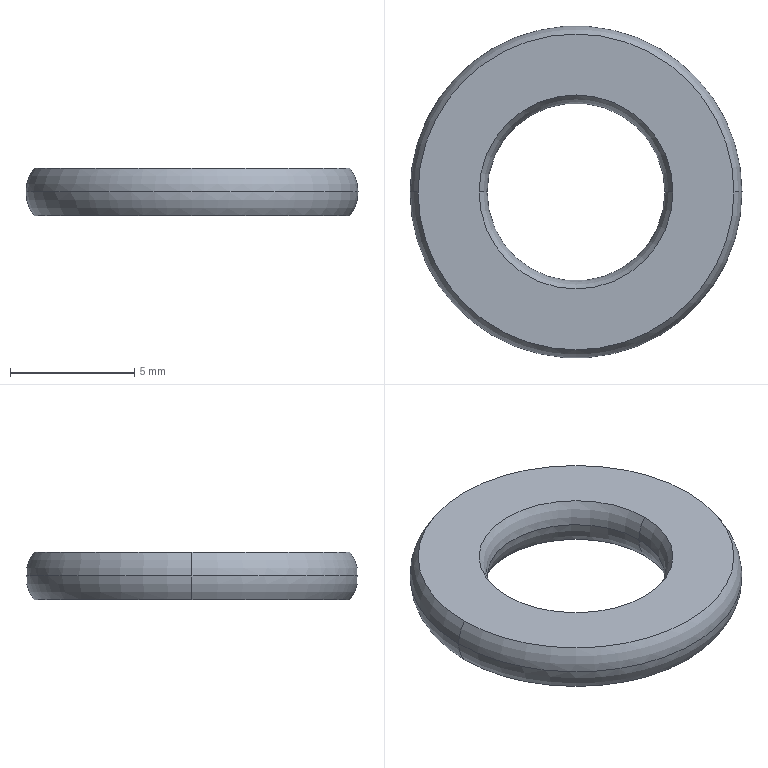Part | Creo | 1 solid | 10 faces | box 13.35 x 13.35 x 1.9 mm | volume 177.011 mm3 | torus 8 | plane 2
STEP:
#1=CARTESIAN_POINT('',(0.,0.,0.));
#2=DIRECTION('',(0.,0.,1.));
#3=DIRECTION('',(1.,0.,0.));
#4=AXIS2_PLACEMENT_3D('',#1,#2,#3);
#5=CARTESIAN_POINT('',(61.1,-29.053,-54.09));
#6=VERTEX_POINT('',#5);
#7=CARTESIAN_POINT('',(68.9,-29.053,-54.09));
#8=VERTEX_POINT('',#7);
#9=CARTESIAN_POINT('',(65.,-29.053,-54.09));
#10=DIRECTION('',(0.,0.,-1.));
#11=DIRECTION('',(-1.,0.,0.));
#12=AXIS2_PLACEMENT_3D('',#9,#10,#11);
#13=CIRCLE('',#12,3.9);
#14=EDGE_CURVE('',#6,#8,#13,.T.);
#15=ORIENTED_EDGE('',*,*,#14,.T.);
#16=CARTESIAN_POINT('',(68.575,-29.053,-55.04));
#17=VERTEX_POINT('',#16);
#18=CARTESIAN_POINT('',(70.125,-29.053,-55.04));
#19=DIRECTION('',(0.,1.,0.));
#20=DIRECTION('',(-1.,0.,0.));
#21=AXIS2_PLACEMENT_3D('',#18,#19,#20);
#22=CIRCLE('',#21,1.55);
#23=EDGE_CURVE('',#17,#8,#22,.T.);
#24=ORIENTED_EDGE('',*,*,#23,.F.);
#25=CARTESIAN_POINT('',(61.425,-29.053,-55.04));
#26=VERTEX_POINT('',#25);
#27=CARTESIAN_POINT('',(65.,-29.053,-55.04));
#28=DIRECTION('',(0.,0.,-1.));
#29=DIRECTION('',(-1.,0.,0.));
#30=AXIS2_PLACEMENT_3D('',#27,#28,#29);
#31=CIRCLE('',#30,3.575);
#32=EDGE_CURVE('',#26,#17,#31,.T.);
#33=ORIENTED_EDGE('',*,*,#32,.F.);
#34=CARTESIAN_POINT('',(59.875,-29.053,-55.04));
#35=DIRECTION('',(0.,-1.,0.));
#36=DIRECTION('',(1.,0.,0.));
#37=AXIS2_PLACEMENT_3D('',#34,#35,#36);
#38=CIRCLE('',#37,1.55);
#39=EDGE_CURVE('',#26,#6,#38,.T.);
#40=ORIENTED_EDGE('',*,*,#39,.T.);
#41=EDGE_LOOP('',(#15,#24,#33,#40));
#42=FACE_OUTER_BOUND('',#41,.F.);
#43=CARTESIAN_POINT('',(65.,-29.053,-55.04));
#44=DIRECTION('',(0.,0.,-1.));
#45=DIRECTION('',(-1.,0.,0.));
#46=AXIS2_PLACEMENT_3D('',#43,#44,#45);
#47=TOROIDAL_SURFACE('',#46,5.125,1.55);
#48=ADVANCED_FACE('',(#42),#47,.T.);
#49=CARTESIAN_POINT('',(58.65,-29.053,-54.09));
#50=VERTEX_POINT('',#49);
#51=CARTESIAN_POINT('',(71.35,-29.053,-54.09));
#52=VERTEX_POINT('',#51);
#53=CARTESIAN_POINT('',(65.,-29.053,-54.09));
#54=DIRECTION('',(0.,0.,1.));
#55=DIRECTION('',(-1.,0.,0.));
#56=AXIS2_PLACEMENT_3D('',#53,#54,#55);
#57=CIRCLE('',#56,6.35);
#58=EDGE_CURVE('',#50,#52,#57,.T.);
#59=ORIENTED_EDGE('',*,*,#58,.F.);
#60=CARTESIAN_POINT('',(65.,-29.053,-54.09));
#61=DIRECTION('',(0.,0.,1.));
#62=DIRECTION('',(1.,0.,0.));
#63=AXIS2_PLACEMENT_3D('',#60,#61,#62);
#64=CIRCLE('',#63,6.35);
#65=EDGE_CURVE('',#52,#50,#64,.T.);
#66=ORIENTED_EDGE('',*,*,#65,.F.);
#67=EDGE_LOOP('',(#59,#66));
#68=FACE_OUTER_BOUND('',#67,.F.);
#69=ORIENTED_EDGE('',*,*,#14,.F.);
#70=CARTESIAN_POINT('',(65.,-29.053,-54.09));
#71=DIRECTION('',(0.,0.,-1.));
#72=DIRECTION('',(1.,0.,0.));
#73=AXIS2_PLACEMENT_3D('',#70,#71,#72);
#74=CIRCLE('',#73,3.9);
#75=EDGE_CURVE('',#8,#6,#74,.T.);
#76=ORIENTED_EDGE('',*,*,#75,.F.);
#77=EDGE_LOOP('',(#69,#76));
#78=FACE_BOUND('',#77,.F.);
#79=CARTESIAN_POINT('',(65.,-22.703,-54.09));
#80=DIRECTION('',(0.,0.,1.));
#81=DIRECTION('',(1.,0.,0.));
#82=AXIS2_PLACEMENT_3D('',#79,#80,#81);
#83=PLANE('',#82);
#84=ADVANCED_FACE('',(#68,#78),#83,.T.);
#85=ORIENTED_EDGE('',*,*,#75,.T.);
#86=ORIENTED_EDGE('',*,*,#39,.F.);
#87=CARTESIAN_POINT('',(65.,-29.053,-55.04));
#88=DIRECTION('',(0.,0.,-1.));
#89=DIRECTION('',(1.,0.,0.));
#90=AXIS2_PLACEMENT_3D('',#87,#88,#89);
#91=CIRCLE('',#90,3.575);
#92=EDGE_CURVE('',#17,#26,#91,.T.);
#93=ORIENTED_EDGE('',*,*,#92,.F.);
#94=ORIENTED_EDGE('',*,*,#23,.T.);
#95=EDGE_LOOP('',(#85,#86,#93,#94));
#96=FACE_OUTER_BOUND('',#95,.F.);
#97=CARTESIAN_POINT('',(65.,-29.053,-55.04));
#98=DIRECTION('',(0.,0.,-1.));
#99=DIRECTION('',(-1.,0.,0.));
#100=AXIS2_PLACEMENT_3D('',#97,#98,#99);
#101=TOROIDAL_SURFACE('',#100,5.125,1.55);
#102=ADVANCED_FACE('',(#96),#101,.T.);
#103=CARTESIAN_POINT('',(61.1,-29.053,-55.99));
#104=VERTEX_POINT('',#103);
#105=CARTESIAN_POINT('',(68.9,-29.053,-55.99));
#106=VERTEX_POINT('',#105);
#107=CARTESIAN_POINT('',(65.,-29.053,-55.99));
#108=DIRECTION('',(0.,0.,1.));
#109=DIRECTION('',(-1.,0.,0.));
#110=AXIS2_PLACEMENT_3D('',#107,#108,#109);
#111=CIRCLE('',#110,3.9);
#112=EDGE_CURVE('',#104,#106,#111,.T.);
#113=ORIENTED_EDGE('',*,*,#112,.T.);
#114=CARTESIAN_POINT('',(70.125,-29.053,-55.04));
#115=DIRECTION('',(0.,1.,0.));
#116=DIRECTION('',(-0.7902,0.,-0.6129));
#117=AXIS2_PLACEMENT_3D('',#114,#115,#116);
#118=CIRCLE('',#117,1.55);
#119=EDGE_CURVE('',#106,#17,#118,.T.);
#120=ORIENTED_EDGE('',*,*,#119,.T.);
#121=ORIENTED_EDGE('',*,*,#92,.T.);
#122=CARTESIAN_POINT('',(59.875,-29.053,-55.04));
#123=DIRECTION('',(0.,-1.,0.));
#124=DIRECTION('',(0.7902,0.,-0.6129));
#125=AXIS2_PLACEMENT_3D('',#122,#123,#124);
#126=CIRCLE('',#125,1.55);
#127=EDGE_CURVE('',#104,#26,#126,.T.);
#128=ORIENTED_EDGE('',*,*,#127,.F.);
#129=EDGE_LOOP('',(#113,#120,#121,#128));
#130=FACE_OUTER_BOUND('',#129,.F.);
#131=CARTESIAN_POINT('',(65.,-29.053,-55.04));
#132=DIRECTION('',(0.,0.,-1.));
#133=DIRECTION('',(-1.,0.,0.));
#134=AXIS2_PLACEMENT_3D('',#131,#132,#133);
#135=TOROIDAL_SURFACE('',#134,5.125,1.55);
#136=ADVANCED_FACE('',(#130),#135,.T.);
#137=CARTESIAN_POINT('',(58.65,-29.053,-55.99));
#138=VERTEX_POINT('',#137);
#139=CARTESIAN_POINT('',(71.35,-29.053,-55.99));
#140=VERTEX_POINT('',#139);
#141=CARTESIAN_POINT('',(65.,-29.053,-55.99));
#142=DIRECTION('',(0.,0.,-1.));
#143=DIRECTION('',(-1.,0.,0.));
#144=AXIS2_PLACEMENT_3D('',#141,#142,#143);
#145=CIRCLE('',#144,6.35);
#146=EDGE_CURVE('',#138,#140,#145,.T.);
#147=ORIENTED_EDGE('',*,*,#146,.F.);
#148=CARTESIAN_POINT('',(65.,-29.053,-55.99));
#149=DIRECTION('',(0.,0.,-1.));
#150=DIRECTION('',(1.,0.,0.));
#151=AXIS2_PLACEMENT_3D('',#148,#149,#150);
#152=CIRCLE('',#151,6.35);
#153=EDGE_CURVE('',#140,#138,#152,.T.);
#154=ORIENTED_EDGE('',*,*,#153,.F.);
#155=EDGE_LOOP('',(#147,#154));
#156=FACE_OUTER_BOUND('',#155,.F.);
#157=ORIENTED_EDGE('',*,*,#112,.F.);
#158=CARTESIAN_POINT('',(65.,-29.053,-55.99));
#159=DIRECTION('',(0.,0.,1.));
#160=DIRECTION('',(1.,0.,0.));
#161=AXIS2_PLACEMENT_3D('',#158,#159,#160);
#162=CIRCLE('',#161,3.9);
#163=EDGE_CURVE('',#106,#104,#162,.T.);
#164=ORIENTED_EDGE('',*,*,#163,.F.);
#165=EDGE_LOOP('',(#157,#164));
#166=FACE_BOUND('',#165,.F.);
#167=CARTESIAN_POINT('',(65.,-25.153,-55.99));
#168=DIRECTION('',(0.,0.,-1.));
#169=DIRECTION('',(-1.,0.,0.));
#170=AXIS2_PLACEMENT_3D('',#167,#168,#169);
#171=PLANE('',#170);
#172=ADVANCED_FACE('',(#156,#166),#171,.T.);
#173=ORIENTED_EDGE('',*,*,#146,.T.);
#174=CARTESIAN_POINT('',(71.675,-29.053,-55.04));
#175=VERTEX_POINT('',#174);
#176=CARTESIAN_POINT('',(70.125,-29.053,-55.04));
#177=DIRECTION('',(0.,1.,0.));
#178=DIRECTION('',(1.,0.,0.));
#179=AXIS2_PLACEMENT_3D('',#176,#177,#178);
#180=CIRCLE('',#179,1.55);
#181=EDGE_CURVE('',#175,#140,#180,.T.);
#182=ORIENTED_EDGE('',*,*,#181,.F.);
#183=CARTESIAN_POINT('',(58.325,-29.053,-55.04));
#184=VERTEX_POINT('',#183);
#185=CARTESIAN_POINT('',(65.,-29.053,-55.04));
#186=DIRECTION('',(0.,0.,-1.));
#187=DIRECTION('',(-1.,0.,0.));
#188=AXIS2_PLACEMENT_3D('',#185,#186,#187);
#189=CIRCLE('',#188,6.675);
#190=EDGE_CURVE('',#184,#175,#189,.T.);
#191=ORIENTED_EDGE('',*,*,#190,.F.);
#192=CARTESIAN_POINT('',(59.875,-29.053,-55.04));
#193=DIRECTION('',(0.,-1.,0.));
#194=DIRECTION('',(-1.,0.,0.));
#195=AXIS2_PLACEMENT_3D('',#192,#193,#194);
#196=CIRCLE('',#195,1.55);
#197=EDGE_CURVE('',#184,#138,#196,.T.);
#198=ORIENTED_EDGE('',*,*,#197,.T.);
#199=EDGE_LOOP('',(#173,#182,#191,#198));
#200=FACE_OUTER_BOUND('',#199,.F.);
#201=CARTESIAN_POINT('',(65.,-29.053,-55.04));
#202=DIRECTION('',(0.,0.,-1.));
#203=DIRECTION('',(-1.,0.,0.));
#204=AXIS2_PLACEMENT_3D('',#201,#202,#203);
#205=TOROIDAL_SURFACE('',#204,5.125,1.55);
#206=ADVANCED_FACE('',(#200),#205,.T.);
#207=ORIENTED_EDGE('',*,*,#153,.T.);
#208=ORIENTED_EDGE('',*,*,#197,.F.);
#209=CARTESIAN_POINT('',(65.,-29.053,-55.04));
#210=DIRECTION('',(0.,0.,-1.));
#211=DIRECTION('',(1.,0.,0.));
#212=AXIS2_PLACEMENT_3D('',#209,#210,#211);
#213=CIRCLE('',#212,6.675);
#214=EDGE_CURVE('',#175,#184,#213,.T.);
#215=ORIENTED_EDGE('',*,*,#214,.F.);
#216=ORIENTED_EDGE('',*,*,#181,.T.);
#217=EDGE_LOOP('',(#207,#208,#215,#216));
#218=FACE_OUTER_BOUND('',#217,.F.);
#219=CARTESIAN_POINT('',(65.,-29.053,-55.04));
#220=DIRECTION('',(0.,0.,-1.));
#221=DIRECTION('',(-1.,0.,0.));
#222=AXIS2_PLACEMENT_3D('',#219,#220,#221);
#223=TOROIDAL_SURFACE('',#222,5.125,1.55);
#224=ADVANCED_FACE('',(#218),#223,.T.);
#225=ORIENTED_EDGE('',*,*,#58,.T.);
#226=CARTESIAN_POINT('',(70.125,-29.053,-55.04));
#227=DIRECTION('',(0.,1.,0.));
#228=DIRECTION('',(0.7902,0.,0.6129));
#229=AXIS2_PLACEMENT_3D('',#226,#227,#228);
#230=CIRCLE('',#229,1.55);
#231=EDGE_CURVE('',#52,#175,#230,.T.);
#232=ORIENTED_EDGE('',*,*,#231,.T.);
#233=ORIENTED_EDGE('',*,*,#214,.T.);
#234=CARTESIAN_POINT('',(59.875,-29.053,-55.04));
#235=DIRECTION('',(0.,-1.,0.));
#236=DIRECTION('',(-0.7902,0.,0.6129));
#237=AXIS2_PLACEMENT_3D('',#234,#235,#236);
#238=CIRCLE('',#237,1.55);
#239=EDGE_CURVE('',#50,#184,#238,.T.);
#240=ORIENTED_EDGE('',*,*,#239,.F.);
#241=EDGE_LOOP('',(#225,#232,#233,#240));
#242=FACE_OUTER_BOUND('',#241,.F.);
#243=CARTESIAN_POINT('',(65.,-29.053,-55.04));
#244=DIRECTION('',(0.,0.,-1.));
#245=DIRECTION('',(-1.,0.,0.));
#246=AXIS2_PLACEMENT_3D('',#243,#244,#245);
#247=TOROIDAL_SURFACE('',#246,5.125,1.55);
#248=ADVANCED_FACE('',(#242),#247,.T.);
#249=ORIENTED_EDGE('',*,*,#65,.T.);
#250=ORIENTED_EDGE('',*,*,#239,.T.);
#251=ORIENTED_EDGE('',*,*,#190,.T.);
#252=ORIENTED_EDGE('',*,*,#231,.F.);
#253=EDGE_LOOP('',(#249,#250,#251,#252));
#254=FACE_OUTER_BOUND('',#253,.F.);
#255=CARTESIAN_POINT('',(65.,-29.053,-55.04));
#256=DIRECTION('',(0.,0.,-1.));
#257=DIRECTION('',(-1.,0.,0.));
#258=AXIS2_PLACEMENT_3D('',#255,#256,#257);
#259=TOROIDAL_SURFACE('',#258,5.125,1.55);
#260=ADVANCED_FACE('',(#254),#259,.T.);
#261=ORIENTED_EDGE('',*,*,#163,.T.);
#262=ORIENTED_EDGE('',*,*,#127,.T.);
#263=ORIENTED_EDGE('',*,*,#32,.T.);
#264=ORIENTED_EDGE('',*,*,#119,.F.);
#265=EDGE_LOOP('',(#261,#262,#263,#264));
#266=FACE_OUTER_BOUND('',#265,.F.);
#267=CARTESIAN_POINT('',(65.,-29.053,-55.04));
#268=DIRECTION('',(0.,0.,-1.));
#269=DIRECTION('',(-1.,0.,0.));
#270=AXIS2_PLACEMENT_3D('',#267,#268,#269);
#271=TOROIDAL_SURFACE('',#270,5.125,1.55);
#272=ADVANCED_FACE('',(#266),#271,.T.);
#273=CLOSED_SHELL('',(#48,#84,#102,#136,#172,#206,#224,#248,#260,#272));
#274=MANIFOLD_SOLID_BREP('',#273);
#275=(LENGTH_UNIT()NAMED_UNIT(*)SI_UNIT(.MILLI.,.METRE.));
#276=UNCERTAINTY_MEASURE_WITH_UNIT(LENGTH_MEASURE(0.001897),#275,'','');
#277=(NAMED_UNIT(*)PLANE_ANGLE_UNIT()SI_UNIT($,.RADIAN.));
#278=PLANE_ANGLE_MEASURE_WITH_UNIT(PLANE_ANGLE_MEASURE(0.01745),#277);
#279=(CONVERSION_BASED_UNIT('DEGREE',#278)NAMED_UNIT(*)PLANE_ANGLE_UNIT());
#280=(NAMED_UNIT(*)SI_UNIT($,.STERADIAN.)SOLID_ANGLE_UNIT());
#281=(GEOMETRIC_REPRESENTATION_CONTEXT(3)GLOBAL_UNCERTAINTY_ASSIGNED_CONTEXT((#276))GLOBAL_UNIT_ASSIGNED_CONTEXT((#275,#279,#280))REPRESENTATION_CONTEXT('',''));
#282=ADVANCED_BREP_SHAPE_REPRESENTATION('',(#4,#274),#281);